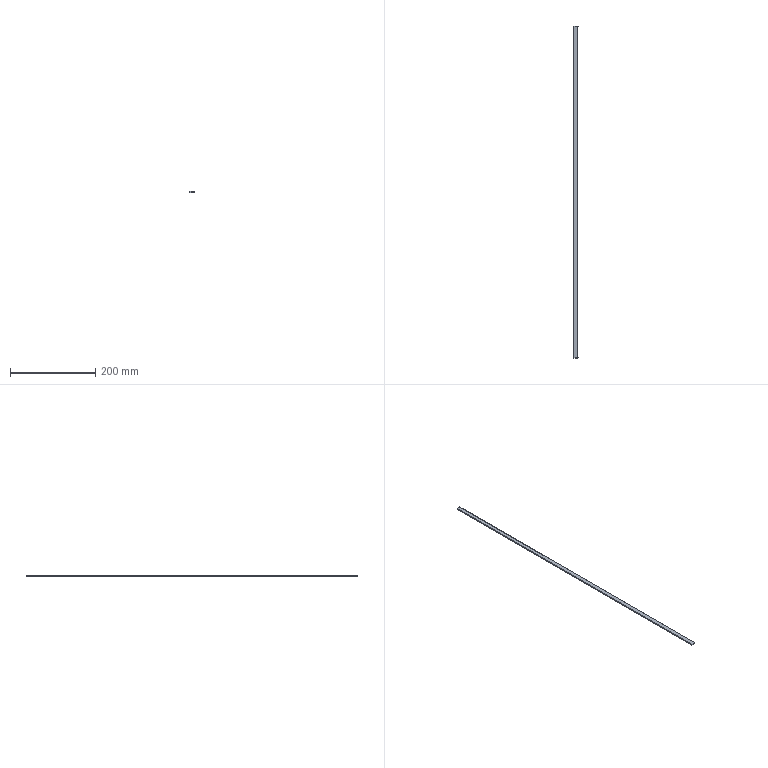Part | SolidWorks | features FlatPattern 1, Hem 1, SMBaseFlange 1, SheetMetal 1 | 1 solid | 14 faces | box 10 x 777 x 2.7 mm | volume 18327 mm3 | plane 12 | cylinder 2 | commonest cylinder face diameters 0.3 x1 2.7 x1
STEP:
#1=CARTESIAN_POINT('',(-1.495,205.207,0.));
#2=VERTEX_POINT('',#1);
#3=CARTESIAN_POINT('',(-10.145,205.207,0.));
#4=VERTEX_POINT('',#3);
#5=CARTESIAN_POINT('',(-10.145,205.207,0.));
#6=DIRECTION('',(-1.,0.,0.));
#7=VECTOR('',#6,1000.);
#8=LINE('',#5,#7);
#9=EDGE_CURVE('',#2,#4,#8,.T.);
#10=ORIENTED_EDGE('',*,*,#9,.F.);
#11=CARTESIAN_POINT('',(-1.495,205.207,-1.2));
#12=VERTEX_POINT('',#11);
#13=CARTESIAN_POINT('',(-1.495,205.207,0.));
#14=DIRECTION('',(0.,0.,-1.));
#15=VECTOR('',#14,1000.);
#16=LINE('',#13,#15);
#17=EDGE_CURVE('',#2,#12,#16,.T.);
#18=ORIENTED_EDGE('',*,*,#17,.T.);
#19=CARTESIAN_POINT('',(-10.145,205.207,-1.2));
#20=VERTEX_POINT('',#19);
#21=CARTESIAN_POINT('',(-10.145,205.207,-1.2));
#22=DIRECTION('',(-1.,0.,0.));
#23=VECTOR('',#22,1000.);
#24=LINE('',#21,#23);
#25=EDGE_CURVE('',#12,#20,#24,.T.);
#26=ORIENTED_EDGE('',*,*,#25,.T.);
#27=CARTESIAN_POINT('',(-10.145,205.207,-1.2));
#28=DIRECTION('',(0.,0.,1.));
#29=VECTOR('',#28,1000.);
#30=LINE('',#27,#29);
#31=EDGE_CURVE('',#20,#4,#30,.T.);
#32=ORIENTED_EDGE('',*,*,#31,.T.);
#33=EDGE_LOOP('',(#10,#18,#26,#32));
#34=FACE_OUTER_BOUND('',#33,.T.);
#35=CARTESIAN_POINT('',(-10.145,205.207,-1.2));
#36=DIRECTION('',(0.,1.,0.));
#37=DIRECTION('',(0.,0.,1.));
#38=AXIS2_PLACEMENT_3D('',#35,#36,#37);
#39=PLANE('',#38);
#40=ADVANCED_FACE('',(#34),#39,.T.);
#41=CARTESIAN_POINT('',(-1.495,-571.793,0.));
#42=VERTEX_POINT('',#41);
#43=CARTESIAN_POINT('',(-1.495,-571.793,-1.2));
#44=VERTEX_POINT('',#43);
#45=CARTESIAN_POINT('',(-1.495,-571.793,0.));
#46=DIRECTION('',(0.,0.,-1.));
#47=VECTOR('',#46,1000.);
#48=LINE('',#45,#47);
#49=EDGE_CURVE('',#42,#44,#48,.T.);
#50=ORIENTED_EDGE('',*,*,#49,.F.);
#51=CARTESIAN_POINT('',(-10.145,-571.793,0.));
#52=VERTEX_POINT('',#51);
#53=CARTESIAN_POINT('',(-10.145,-571.793,0.));
#54=DIRECTION('',(1.,0.,0.));
#55=VECTOR('',#54,1000.);
#56=LINE('',#53,#55);
#57=EDGE_CURVE('',#52,#42,#56,.T.);
#58=ORIENTED_EDGE('',*,*,#57,.F.);
#59=CARTESIAN_POINT('',(-10.145,-571.793,-1.2));
#60=VERTEX_POINT('',#59);
#61=CARTESIAN_POINT('',(-10.145,-571.793,-1.2));
#62=DIRECTION('',(0.,0.,1.));
#63=VECTOR('',#62,1000.);
#64=LINE('',#61,#63);
#65=EDGE_CURVE('',#60,#52,#64,.T.);
#66=ORIENTED_EDGE('',*,*,#65,.F.);
#67=CARTESIAN_POINT('',(-10.145,-571.793,-1.2));
#68=DIRECTION('',(1.,0.,0.));
#69=VECTOR('',#68,1000.);
#70=LINE('',#67,#69);
#71=EDGE_CURVE('',#60,#44,#70,.T.);
#72=ORIENTED_EDGE('',*,*,#71,.T.);
#73=EDGE_LOOP('',(#50,#58,#66,#72));
#74=FACE_OUTER_BOUND('',#73,.T.);
#75=CARTESIAN_POINT('',(-10.145,-571.793,-1.2));
#76=DIRECTION('',(0.,-1.,0.));
#77=DIRECTION('',(0.,0.,-1.));
#78=AXIS2_PLACEMENT_3D('',#75,#76,#77);
#79=PLANE('',#78);
#80=ADVANCED_FACE('',(#74),#79,.T.);
#81=CARTESIAN_POINT('',(-10.145,205.207,0.));
#82=DIRECTION('',(0.,-1.,0.));
#83=VECTOR('',#82,1000.);
#84=LINE('',#81,#83);
#85=EDGE_CURVE('',#4,#52,#84,.T.);
#86=ORIENTED_EDGE('',*,*,#85,.F.);
#87=ORIENTED_EDGE('',*,*,#31,.F.);
#88=CARTESIAN_POINT('',(-10.145,205.207,-1.2));
#89=DIRECTION('',(0.,-1.,0.));
#90=VECTOR('',#89,1000.);
#91=LINE('',#88,#90);
#92=EDGE_CURVE('',#20,#60,#91,.T.);
#93=ORIENTED_EDGE('',*,*,#92,.T.);
#94=ORIENTED_EDGE('',*,*,#65,.T.);
#95=EDGE_LOOP('',(#86,#87,#93,#94));
#96=FACE_OUTER_BOUND('',#95,.T.);
#97=CARTESIAN_POINT('',(-10.145,205.207,-1.2));
#98=DIRECTION('',(-1.,0.,0.));
#99=DIRECTION('',(0.,-1.,0.));
#100=AXIS2_PLACEMENT_3D('',#97,#98,#99);
#101=PLANE('',#100);
#102=ADVANCED_FACE('',(#96),#101,.T.);
#103=ORIENTED_EDGE('',*,*,#25,.F.);
#104=CARTESIAN_POINT('',(-1.495,205.207,-1.2));
#105=DIRECTION('',(0.,-1.,0.));
#106=VECTOR('',#105,1000.);
#107=LINE('',#104,#106);
#108=EDGE_CURVE('',#12,#44,#107,.T.);
#109=ORIENTED_EDGE('',*,*,#108,.T.);
#110=ORIENTED_EDGE('',*,*,#71,.F.);
#111=ORIENTED_EDGE('',*,*,#92,.F.);
#112=EDGE_LOOP('',(#103,#109,#110,#111));
#113=FACE_OUTER_BOUND('',#112,.T.);
#114=CARTESIAN_POINT('',(0.,0.,-1.2));
#115=DIRECTION('',(0.,0.,1.));
#116=DIRECTION('',(1.,0.,0.));
#117=AXIS2_PLACEMENT_3D('',#114,#115,#116);
#118=PLANE('',#117);
#119=ADVANCED_FACE('',(#113),#118,.F.);
#120=CARTESIAN_POINT('',(-1.495,205.207,0.));
#121=DIRECTION('',(0.,-1.,0.));
#122=VECTOR('',#121,1000.);
#123=LINE('',#120,#122);
#124=EDGE_CURVE('',#2,#42,#123,.T.);
#125=ORIENTED_EDGE('',*,*,#124,.F.);
#126=ORIENTED_EDGE('',*,*,#9,.T.);
#127=ORIENTED_EDGE('',*,*,#85,.T.);
#128=ORIENTED_EDGE('',*,*,#57,.T.);
#129=EDGE_LOOP('',(#125,#126,#127,#128));
#130=FACE_OUTER_BOUND('',#129,.T.);
#131=CARTESIAN_POINT('',(0.,0.,0.));
#132=DIRECTION('',(0.,0.,1.));
#133=DIRECTION('',(1.,0.,0.));
#134=AXIS2_PLACEMENT_3D('',#131,#132,#133);
#135=PLANE('',#134);
#136=ADVANCED_FACE('',(#130),#135,.T.);
#137=CARTESIAN_POINT('',(-1.495,205.207,0.3));
#138=VERTEX_POINT('',#137);
#139=CARTESIAN_POINT('',(-1.495,205.207,1.5));
#140=VERTEX_POINT('',#139);
#141=CARTESIAN_POINT('',(-1.495,205.207,1.5));
#142=DIRECTION('',(0.,0.,1.));
#143=VECTOR('',#142,1000.);
#144=LINE('',#141,#143);
#145=EDGE_CURVE('',#138,#140,#144,.T.);
#146=ORIENTED_EDGE('',*,*,#145,.F.);
#147=CARTESIAN_POINT('',(-10.145,205.207,0.3));
#148=VERTEX_POINT('',#147);
#149=CARTESIAN_POINT('',(-5.82,205.207,0.3));
#150=DIRECTION('',(1.,0.,0.));
#151=VECTOR('',#150,1000.);
#152=LINE('',#149,#151);
#153=EDGE_CURVE('',#148,#138,#152,.T.);
#154=ORIENTED_EDGE('',*,*,#153,.F.);
#155=CARTESIAN_POINT('',(-10.145,205.207,1.5));
#156=VERTEX_POINT('',#155);
#157=CARTESIAN_POINT('',(-10.145,205.207,1.5));
#158=DIRECTION('',(0.,0.,1.));
#159=VECTOR('',#158,1000.);
#160=LINE('',#157,#159);
#161=EDGE_CURVE('',#148,#156,#160,.T.);
#162=ORIENTED_EDGE('',*,*,#161,.T.);
#163=CARTESIAN_POINT('',(-5.82,205.207,1.5));
#164=DIRECTION('',(1.,0.,0.));
#165=VECTOR('',#164,1000.);
#166=LINE('',#163,#165);
#167=EDGE_CURVE('',#156,#140,#166,.T.);
#168=ORIENTED_EDGE('',*,*,#167,.T.);
#169=EDGE_LOOP('',(#146,#154,#162,#168));
#170=FACE_OUTER_BOUND('',#169,.T.);
#171=CARTESIAN_POINT('',(-5.82,205.207,1.5));
#172=DIRECTION('',(0.,-1.,0.));
#173=DIRECTION('',(1.,0.,0.));
#174=AXIS2_PLACEMENT_3D('',#171,#172,#173);
#175=PLANE('',#174);
#176=ADVANCED_FACE('',(#170),#175,.F.);
#177=ORIENTED_EDGE('',*,*,#161,.F.);
#178=CARTESIAN_POINT('',(-10.145,-571.793,0.3));
#179=VERTEX_POINT('',#178);
#180=CARTESIAN_POINT('',(-10.145,-183.293,0.3));
#181=DIRECTION('',(0.,1.,0.));
#182=VECTOR('',#181,1000.);
#183=LINE('',#180,#182);
#184=EDGE_CURVE('',#179,#148,#183,.T.);
#185=ORIENTED_EDGE('',*,*,#184,.F.);
#186=CARTESIAN_POINT('',(-10.145,-571.793,1.5));
#187=VERTEX_POINT('',#186);
#188=CARTESIAN_POINT('',(-10.145,-571.793,1.5));
#189=DIRECTION('',(0.,0.,1.));
#190=VECTOR('',#189,1000.);
#191=LINE('',#188,#190);
#192=EDGE_CURVE('',#179,#187,#191,.T.);
#193=ORIENTED_EDGE('',*,*,#192,.T.);
#194=CARTESIAN_POINT('',(-10.145,-183.293,1.5));
#195=DIRECTION('',(0.,1.,0.));
#196=VECTOR('',#195,1000.);
#197=LINE('',#194,#196);
#198=EDGE_CURVE('',#187,#156,#197,.T.);
#199=ORIENTED_EDGE('',*,*,#198,.T.);
#200=EDGE_LOOP('',(#177,#185,#193,#199));
#201=FACE_OUTER_BOUND('',#200,.T.);
#202=CARTESIAN_POINT('',(-10.145,-183.293,1.5));
#203=DIRECTION('',(1.,0.,0.));
#204=DIRECTION('',(0.,1.,0.));
#205=AXIS2_PLACEMENT_3D('',#202,#203,#204);
#206=PLANE('',#205);
#207=ADVANCED_FACE('',(#201),#206,.F.);
#208=CARTESIAN_POINT('',(-1.495,-571.793,0.3));
#209=VERTEX_POINT('',#208);
#210=CARTESIAN_POINT('',(-5.82,-571.793,0.3));
#211=DIRECTION('',(-1.,0.,0.));
#212=VECTOR('',#211,1000.);
#213=LINE('',#210,#212);
#214=EDGE_CURVE('',#209,#179,#213,.T.);
#215=ORIENTED_EDGE('',*,*,#214,.F.);
#216=CARTESIAN_POINT('',(-1.495,-571.793,1.5));
#217=VERTEX_POINT('',#216);
#218=CARTESIAN_POINT('',(-1.495,-571.793,1.5));
#219=DIRECTION('',(0.,0.,1.));
#220=VECTOR('',#219,1000.);
#221=LINE('',#218,#220);
#222=EDGE_CURVE('',#209,#217,#221,.T.);
#223=ORIENTED_EDGE('',*,*,#222,.T.);
#224=CARTESIAN_POINT('',(-5.82,-571.793,1.5));
#225=DIRECTION('',(-1.,0.,0.));
#226=VECTOR('',#225,1000.);
#227=LINE('',#224,#226);
#228=EDGE_CURVE('',#217,#187,#227,.T.);
#229=ORIENTED_EDGE('',*,*,#228,.T.);
#230=ORIENTED_EDGE('',*,*,#192,.F.);
#231=EDGE_LOOP('',(#215,#223,#229,#230));
#232=FACE_OUTER_BOUND('',#231,.T.);
#233=CARTESIAN_POINT('',(-5.82,-571.793,1.5));
#234=DIRECTION('',(0.,1.,0.));
#235=DIRECTION('',(-1.,0.,0.));
#236=AXIS2_PLACEMENT_3D('',#233,#234,#235);
#237=PLANE('',#236);
#238=ADVANCED_FACE('',(#232),#237,.F.);
#239=ORIENTED_EDGE('',*,*,#198,.F.);
#240=ORIENTED_EDGE('',*,*,#228,.F.);
#241=CARTESIAN_POINT('',(-1.495,-183.293,1.5));
#242=DIRECTION('',(0.,-1.,0.));
#243=VECTOR('',#242,1000.);
#244=LINE('',#241,#243);
#245=EDGE_CURVE('',#140,#217,#244,.T.);
#246=ORIENTED_EDGE('',*,*,#245,.F.);
#247=ORIENTED_EDGE('',*,*,#167,.F.);
#248=EDGE_LOOP('',(#239,#240,#246,#247));
#249=FACE_OUTER_BOUND('',#248,.T.);
#250=CARTESIAN_POINT('',(-5.82,-183.293,1.5));
#251=DIRECTION('',(0.,0.,1.));
#252=DIRECTION('',(1.,0.,0.));
#253=AXIS2_PLACEMENT_3D('',#250,#251,#252);
#254=PLANE('',#253);
#255=ADVANCED_FACE('',(#249),#254,.T.);
#256=ORIENTED_EDGE('',*,*,#184,.T.);
#257=ORIENTED_EDGE('',*,*,#153,.T.);
#258=CARTESIAN_POINT('',(-1.495,-183.293,0.3));
#259=DIRECTION('',(0.,-1.,0.));
#260=VECTOR('',#259,1000.);
#261=LINE('',#258,#260);
#262=EDGE_CURVE('',#138,#209,#261,.T.);
#263=ORIENTED_EDGE('',*,*,#262,.T.);
#264=ORIENTED_EDGE('',*,*,#214,.T.);
#265=EDGE_LOOP('',(#256,#257,#263,#264));
#266=FACE_OUTER_BOUND('',#265,.T.);
#267=CARTESIAN_POINT('',(-5.82,-183.293,0.3));
#268=DIRECTION('',(0.,0.,1.));
#269=DIRECTION('',(1.,0.,0.));
#270=AXIS2_PLACEMENT_3D('',#267,#268,#269);
#271=PLANE('',#270);
#272=ADVANCED_FACE('',(#266),#271,.F.);
#273=ORIENTED_EDGE('',*,*,#222,.F.);
#274=CARTESIAN_POINT('',(-1.495,-571.793,0.15));
#275=DIRECTION('',(0.,-1.,0.));
#276=DIRECTION('',(0.,0.,1.));
#277=AXIS2_PLACEMENT_3D('',#274,#275,#276);
#278=CIRCLE('',#277,0.15);
#279=EDGE_CURVE('',#42,#209,#278,.T.);
#280=ORIENTED_EDGE('',*,*,#279,.F.);
#281=ORIENTED_EDGE('',*,*,#49,.T.);
#282=CARTESIAN_POINT('',(-1.495,-571.793,0.15));
#283=DIRECTION('',(0.,-1.,0.));
#284=DIRECTION('',(0.,0.,1.));
#285=AXIS2_PLACEMENT_3D('',#282,#283,#284);
#286=CIRCLE('',#285,1.35);
#287=EDGE_CURVE('',#44,#217,#286,.T.);
#288=ORIENTED_EDGE('',*,*,#287,.T.);
#289=EDGE_LOOP('',(#273,#280,#281,#288));
#290=FACE_OUTER_BOUND('',#289,.T.);
#291=CARTESIAN_POINT('',(-1.495,-571.793,0.15));
#292=DIRECTION('',(0.,-1.,0.));
#293=DIRECTION('',(0.,0.,-1.));
#294=AXIS2_PLACEMENT_3D('',#291,#292,#293);
#295=PLANE('',#294);
#296=ADVANCED_FACE('',(#290),#295,.T.);
#297=CARTESIAN_POINT('',(-1.495,205.207,0.15));
#298=DIRECTION('',(0.,1.,0.));
#299=DIRECTION('',(0.,0.,1.));
#300=AXIS2_PLACEMENT_3D('',#297,#298,#299);
#301=CIRCLE('',#300,0.15);
#302=EDGE_CURVE('',#138,#2,#301,.T.);
#303=ORIENTED_EDGE('',*,*,#302,.F.);
#304=ORIENTED_EDGE('',*,*,#145,.T.);
#305=CARTESIAN_POINT('',(-1.495,205.207,0.15));
#306=DIRECTION('',(0.,1.,0.));
#307=DIRECTION('',(0.,0.,1.));
#308=AXIS2_PLACEMENT_3D('',#305,#306,#307);
#309=CIRCLE('',#308,1.35);
#310=EDGE_CURVE('',#140,#12,#309,.T.);
#311=ORIENTED_EDGE('',*,*,#310,.T.);
#312=ORIENTED_EDGE('',*,*,#17,.F.);
#313=EDGE_LOOP('',(#303,#304,#311,#312));
#314=FACE_OUTER_BOUND('',#313,.T.);
#315=CARTESIAN_POINT('',(-1.495,205.207,0.15));
#316=DIRECTION('',(0.,-1.,0.));
#317=DIRECTION('',(0.,0.,-1.));
#318=AXIS2_PLACEMENT_3D('',#315,#316,#317);
#319=PLANE('',#318);
#320=ADVANCED_FACE('',(#314),#319,.F.);
#321=ORIENTED_EDGE('',*,*,#108,.F.);
#322=ORIENTED_EDGE('',*,*,#310,.F.);
#323=ORIENTED_EDGE('',*,*,#245,.T.);
#324=ORIENTED_EDGE('',*,*,#287,.F.);
#325=EDGE_LOOP('',(#321,#322,#323,#324));
#326=FACE_OUTER_BOUND('',#325,.T.);
#327=CARTESIAN_POINT('',(-1.495,205.207,0.15));
#328=DIRECTION('',(0.,1.,0.));
#329=DIRECTION('',(0.,0.,1.));
#330=AXIS2_PLACEMENT_3D('',#327,#328,#329);
#331=CYLINDRICAL_SURFACE('',#330,1.35);
#332=ADVANCED_FACE('',(#326),#331,.T.);
#333=ORIENTED_EDGE('',*,*,#124,.T.);
#334=ORIENTED_EDGE('',*,*,#279,.T.);
#335=ORIENTED_EDGE('',*,*,#262,.F.);
#336=ORIENTED_EDGE('',*,*,#302,.T.);
#337=EDGE_LOOP('',(#333,#334,#335,#336));
#338=FACE_OUTER_BOUND('',#337,.T.);
#339=CARTESIAN_POINT('',(-1.495,205.207,0.15));
#340=DIRECTION('',(0.,1.,0.));
#341=DIRECTION('',(0.,0.,1.));
#342=AXIS2_PLACEMENT_3D('',#339,#340,#341);
#343=CYLINDRICAL_SURFACE('',#342,0.15);
#344=ADVANCED_FACE('',(#338),#343,.F.);
#345=CLOSED_SHELL('',(#40,#80,#102,#119,#136,#176,#207,#238,#255,#272,#296,#320,#332,#344));
#346=MANIFOLD_SOLID_BREP('',#345);
#347=CARTESIAN_POINT('',(0.,0.,0.));
#348=DIRECTION('',(0.,0.,1.));
#349=DIRECTION('',(1.,0.,0.));
#350=AXIS2_PLACEMENT_3D('',#347,#348,#349);
#351=(LENGTH_UNIT()NAMED_UNIT(*)SI_UNIT(.MILLI.,.METRE.));
#352=UNCERTAINTY_MEASURE_WITH_UNIT(LENGTH_MEASURE(0.00001),#351,'','');
#353=(NAMED_UNIT(*)PLANE_ANGLE_UNIT()SI_UNIT($,.RADIAN.));
#354=(NAMED_UNIT(*)SI_UNIT($,.STERADIAN.)SOLID_ANGLE_UNIT());
#355=(GEOMETRIC_REPRESENTATION_CONTEXT(3)GLOBAL_UNCERTAINTY_ASSIGNED_CONTEXT((#352))GLOBAL_UNIT_ASSIGNED_CONTEXT((#351,#353,#354))REPRESENTATION_CONTEXT('',''));
#356=ADVANCED_BREP_SHAPE_REPRESENTATION('',(#346,#350),#355);